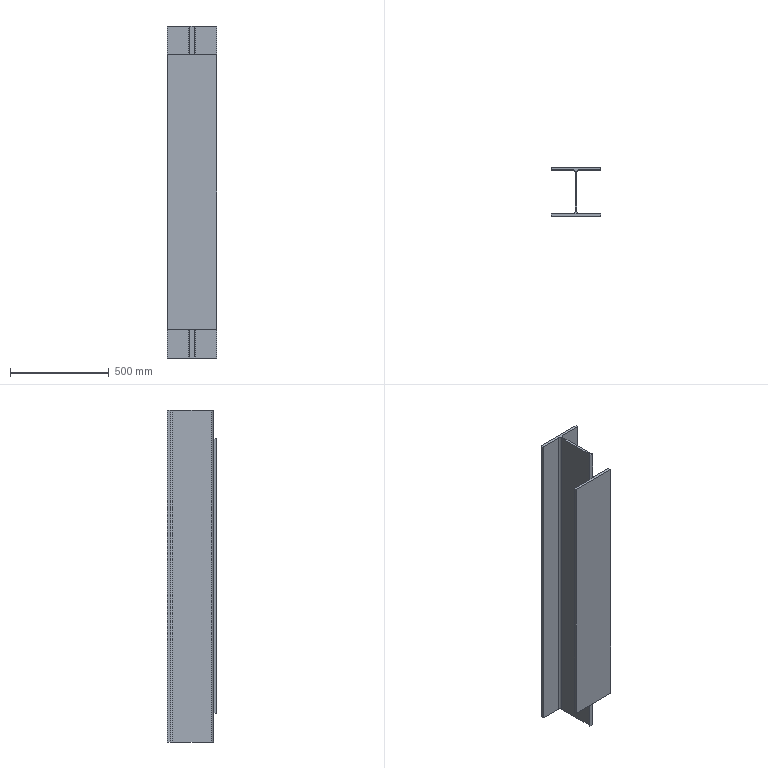Part | SolidWorks | features Extrusion 1, ICE 1 | 1 solid | 22 faces | box 250 x 250 x 1681 mm | volume 14328994 mm3 | plane 18 | cylinder 4 | commonest cylinder face diameters 26 x4
STEP:
#1=CARTESIAN_POINT('',(135.572,16.,0.));
#2=VERTEX_POINT('',#1);
#3=CARTESIAN_POINT('',(129.5,27.,0.));
#4=VERTEX_POINT('',#3);
#5=CARTESIAN_POINT('',(142.5,27.,0.));
#6=DIRECTION('',(0.,0.,-1.));
#7=DIRECTION('',(-1.,0.,0.));
#8=AXIS2_PLACEMENT_3D('',#5,#6,#7);
#9=CIRCLE('',#8,13.);
#10=EDGE_CURVE('',#2,#4,#9,.T.);
#11=ORIENTED_EDGE('',*,*,#10,.F.);
#12=CARTESIAN_POINT('',(114.428,16.,0.));
#13=VERTEX_POINT('',#12);
#14=CARTESIAN_POINT('',(142.5,16.,0.));
#15=DIRECTION('',(-1.,0.,0.));
#16=VECTOR('',#15,1000.);
#17=LINE('',#14,#16);
#18=EDGE_CURVE('',#2,#13,#17,.T.);
#19=ORIENTED_EDGE('',*,*,#18,.T.);
#20=CARTESIAN_POINT('',(120.5,27.,0.));
#21=VERTEX_POINT('',#20);
#22=CARTESIAN_POINT('',(107.5,27.,0.));
#23=DIRECTION('',(0.,0.,-1.));
#24=DIRECTION('',(-1.,0.,0.));
#25=AXIS2_PLACEMENT_3D('',#22,#23,#24);
#26=CIRCLE('',#25,13.);
#27=EDGE_CURVE('',#21,#13,#26,.T.);
#28=ORIENTED_EDGE('',*,*,#27,.F.);
#29=CARTESIAN_POINT('',(120.5,223.,0.));
#30=VERTEX_POINT('',#29);
#31=CARTESIAN_POINT('',(120.5,223.,0.));
#32=DIRECTION('',(0.,-1.,0.));
#33=VECTOR('',#32,1000.);
#34=LINE('',#31,#33);
#35=EDGE_CURVE('',#30,#21,#34,.T.);
#36=ORIENTED_EDGE('',*,*,#35,.F.);
#37=CARTESIAN_POINT('',(107.5,236.,0.));
#38=VERTEX_POINT('',#37);
#39=CARTESIAN_POINT('',(107.5,223.,0.));
#40=DIRECTION('',(0.,0.,-1.));
#41=DIRECTION('',(-1.,0.,0.));
#42=AXIS2_PLACEMENT_3D('',#39,#40,#41);
#43=CIRCLE('',#42,13.);
#44=EDGE_CURVE('',#38,#30,#43,.T.);
#45=ORIENTED_EDGE('',*,*,#44,.F.);
#46=CARTESIAN_POINT('',(0.,236.,0.));
#47=VERTEX_POINT('',#46);
#48=CARTESIAN_POINT('',(0.,236.,0.));
#49=DIRECTION('',(1.,0.,0.));
#50=VECTOR('',#49,1000.);
#51=LINE('',#48,#50);
#52=EDGE_CURVE('',#47,#38,#51,.T.);
#53=ORIENTED_EDGE('',*,*,#52,.F.);
#54=CARTESIAN_POINT('',(0.,250.,0.));
#55=VERTEX_POINT('',#54);
#56=CARTESIAN_POINT('',(0.,250.,0.));
#57=DIRECTION('',(0.,-1.,0.));
#58=VECTOR('',#57,1000.);
#59=LINE('',#56,#58);
#60=EDGE_CURVE('',#55,#47,#59,.T.);
#61=ORIENTED_EDGE('',*,*,#60,.F.);
#62=CARTESIAN_POINT('',(250.,250.,0.));
#63=VERTEX_POINT('',#62);
#64=CARTESIAN_POINT('',(250.,250.,0.));
#65=DIRECTION('',(-1.,0.,0.));
#66=VECTOR('',#65,1000.);
#67=LINE('',#64,#66);
#68=EDGE_CURVE('',#63,#55,#67,.T.);
#69=ORIENTED_EDGE('',*,*,#68,.F.);
#70=CARTESIAN_POINT('',(250.,236.,0.));
#71=VERTEX_POINT('',#70);
#72=CARTESIAN_POINT('',(250.,236.,0.));
#73=DIRECTION('',(0.,1.,0.));
#74=VECTOR('',#73,1000.);
#75=LINE('',#72,#74);
#76=EDGE_CURVE('',#71,#63,#75,.T.);
#77=ORIENTED_EDGE('',*,*,#76,.F.);
#78=CARTESIAN_POINT('',(142.5,236.,0.));
#79=VERTEX_POINT('',#78);
#80=CARTESIAN_POINT('',(142.5,236.,0.));
#81=DIRECTION('',(1.,0.,0.));
#82=VECTOR('',#81,1000.);
#83=LINE('',#80,#82);
#84=EDGE_CURVE('',#79,#71,#83,.T.);
#85=ORIENTED_EDGE('',*,*,#84,.F.);
#86=CARTESIAN_POINT('',(129.5,223.,0.));
#87=VERTEX_POINT('',#86);
#88=CARTESIAN_POINT('',(142.5,223.,0.));
#89=DIRECTION('',(0.,0.,-1.));
#90=DIRECTION('',(-1.,0.,0.));
#91=AXIS2_PLACEMENT_3D('',#88,#89,#90);
#92=CIRCLE('',#91,13.);
#93=EDGE_CURVE('',#87,#79,#92,.T.);
#94=ORIENTED_EDGE('',*,*,#93,.F.);
#95=CARTESIAN_POINT('',(129.5,27.,0.));
#96=DIRECTION('',(0.,1.,0.));
#97=VECTOR('',#96,1000.);
#98=LINE('',#95,#97);
#99=EDGE_CURVE('',#4,#87,#98,.T.);
#100=ORIENTED_EDGE('',*,*,#99,.F.);
#101=EDGE_LOOP('',(#11,#19,#28,#36,#45,#53,#61,#69,#77,#85,#94,#100));
#102=FACE_OUTER_BOUND('',#101,.T.);
#103=CARTESIAN_POINT('',(142.5,27.,0.));
#104=DIRECTION('',(0.,0.,-1.));
#105=DIRECTION('',(-1.,0.,0.));
#106=AXIS2_PLACEMENT_3D('',#103,#104,#105);
#107=PLANE('',#106);
#108=ADVANCED_FACE('',(#102),#107,.T.);
#109=CARTESIAN_POINT('',(0.,14.,1534.5));
#110=VERTEX_POINT('',#109);
#111=CARTESIAN_POINT('',(0.,14.,146.5));
#112=VERTEX_POINT('',#111);
#113=CARTESIAN_POINT('',(0.,14.,1681.));
#114=DIRECTION('',(0.,0.,-1.));
#115=VECTOR('',#114,1000.);
#116=LINE('',#113,#115);
#117=EDGE_CURVE('',#110,#112,#116,.T.);
#118=ORIENTED_EDGE('',*,*,#117,.T.);
#119=CARTESIAN_POINT('',(0.,0.,146.5));
#120=VERTEX_POINT('',#119);
#121=CARTESIAN_POINT('',(0.,16.,146.5));
#122=DIRECTION('',(0.,-1.,0.));
#123=VECTOR('',#122,1000.);
#124=LINE('',#121,#123);
#125=EDGE_CURVE('',#112,#120,#124,.T.);
#126=ORIENTED_EDGE('',*,*,#125,.T.);
#127=CARTESIAN_POINT('',(0.,0.,1534.5));
#128=VERTEX_POINT('',#127);
#129=CARTESIAN_POINT('',(0.,0.,1681.));
#130=DIRECTION('',(0.,0.,-1.));
#131=VECTOR('',#130,1000.);
#132=LINE('',#129,#131);
#133=EDGE_CURVE('',#128,#120,#132,.T.);
#134=ORIENTED_EDGE('',*,*,#133,.F.);
#135=CARTESIAN_POINT('',(0.,16.,1534.5));
#136=DIRECTION('',(0.,-1.,0.));
#137=VECTOR('',#136,1000.);
#138=LINE('',#135,#137);
#139=EDGE_CURVE('',#110,#128,#138,.T.);
#140=ORIENTED_EDGE('',*,*,#139,.F.);
#141=EDGE_LOOP('',(#118,#126,#134,#140));
#142=FACE_OUTER_BOUND('',#141,.T.);
#143=CARTESIAN_POINT('',(0.,14.,1681.));
#144=DIRECTION('',(1.,0.,0.));
#145=DIRECTION('',(0.,1.,0.));
#146=AXIS2_PLACEMENT_3D('',#143,#144,#145);
#147=PLANE('',#146);
#148=ADVANCED_FACE('',(#142),#147,.F.);
#149=ORIENTED_EDGE('',*,*,#133,.T.);
#150=CARTESIAN_POINT('',(250.,0.,146.5));
#151=VERTEX_POINT('',#150);
#152=CARTESIAN_POINT('',(250.,0.,146.5));
#153=DIRECTION('',(-1.,0.,0.));
#154=VECTOR('',#153,1000.);
#155=LINE('',#152,#154);
#156=EDGE_CURVE('',#151,#120,#155,.T.);
#157=ORIENTED_EDGE('',*,*,#156,.F.);
#158=CARTESIAN_POINT('',(250.,0.,1534.5));
#159=VERTEX_POINT('',#158);
#160=CARTESIAN_POINT('',(250.,0.,1681.));
#161=DIRECTION('',(0.,0.,-1.));
#162=VECTOR('',#161,1000.);
#163=LINE('',#160,#162);
#164=EDGE_CURVE('',#159,#151,#163,.T.);
#165=ORIENTED_EDGE('',*,*,#164,.F.);
#166=CARTESIAN_POINT('',(250.,0.,1534.5));
#167=DIRECTION('',(1.,0.,0.));
#168=VECTOR('',#167,1000.);
#169=LINE('',#166,#168);
#170=EDGE_CURVE('',#128,#159,#169,.T.);
#171=ORIENTED_EDGE('',*,*,#170,.F.);
#172=EDGE_LOOP('',(#149,#157,#165,#171));
#173=FACE_OUTER_BOUND('',#172,.T.);
#174=CARTESIAN_POINT('',(0.,0.,1681.));
#175=DIRECTION('',(0.,1.,0.));
#176=DIRECTION('',(-1.,0.,0.));
#177=AXIS2_PLACEMENT_3D('',#174,#175,#176);
#178=PLANE('',#177);
#179=ADVANCED_FACE('',(#173),#178,.F.);
#180=ORIENTED_EDGE('',*,*,#164,.T.);
#181=CARTESIAN_POINT('',(250.,14.,146.5));
#182=VERTEX_POINT('',#181);
#183=CARTESIAN_POINT('',(250.,16.,146.5));
#184=DIRECTION('',(0.,-1.,0.));
#185=VECTOR('',#184,1000.);
#186=LINE('',#183,#185);
#187=EDGE_CURVE('',#182,#151,#186,.T.);
#188=ORIENTED_EDGE('',*,*,#187,.F.);
#189=CARTESIAN_POINT('',(250.,14.,1534.5));
#190=VERTEX_POINT('',#189);
#191=CARTESIAN_POINT('',(250.,14.,1681.));
#192=DIRECTION('',(0.,0.,-1.));
#193=VECTOR('',#192,1000.);
#194=LINE('',#191,#193);
#195=EDGE_CURVE('',#190,#182,#194,.T.);
#196=ORIENTED_EDGE('',*,*,#195,.F.);
#197=CARTESIAN_POINT('',(250.,16.,1534.5));
#198=DIRECTION('',(0.,-1.,0.));
#199=VECTOR('',#198,1000.);
#200=LINE('',#197,#199);
#201=EDGE_CURVE('',#190,#159,#200,.T.);
#202=ORIENTED_EDGE('',*,*,#201,.T.);
#203=EDGE_LOOP('',(#180,#188,#196,#202));
#204=FACE_OUTER_BOUND('',#203,.T.);
#205=CARTESIAN_POINT('',(250.,0.,1681.));
#206=DIRECTION('',(-1.,0.,0.));
#207=DIRECTION('',(0.,0.,1.));
#208=AXIS2_PLACEMENT_3D('',#205,#206,#207);
#209=PLANE('',#208);
#210=ADVANCED_FACE('',(#204),#209,.F.);
#211=ORIENTED_EDGE('',*,*,#195,.T.);
#212=CARTESIAN_POINT('',(142.5,14.,146.5));
#213=VERTEX_POINT('',#212);
#214=CARTESIAN_POINT('',(250.,14.,146.5));
#215=DIRECTION('',(-1.,0.,0.));
#216=VECTOR('',#215,1000.);
#217=LINE('',#214,#216);
#218=EDGE_CURVE('',#182,#213,#217,.T.);
#219=ORIENTED_EDGE('',*,*,#218,.T.);
#220=CARTESIAN_POINT('',(142.5,14.,1534.5));
#221=VERTEX_POINT('',#220);
#222=CARTESIAN_POINT('',(142.5,14.,1681.));
#223=DIRECTION('',(0.,0.,-1.));
#224=VECTOR('',#223,1000.);
#225=LINE('',#222,#224);
#226=EDGE_CURVE('',#221,#213,#225,.T.);
#227=ORIENTED_EDGE('',*,*,#226,.F.);
#228=CARTESIAN_POINT('',(250.,14.,1534.5));
#229=DIRECTION('',(1.,0.,0.));
#230=VECTOR('',#229,1000.);
#231=LINE('',#228,#230);
#232=EDGE_CURVE('',#221,#190,#231,.T.);
#233=ORIENTED_EDGE('',*,*,#232,.T.);
#234=EDGE_LOOP('',(#211,#219,#227,#233));
#235=FACE_OUTER_BOUND('',#234,.T.);
#236=CARTESIAN_POINT('',(250.,14.,1681.));
#237=DIRECTION('',(0.,-1.,0.));
#238=DIRECTION('',(1.,0.,0.));
#239=AXIS2_PLACEMENT_3D('',#236,#237,#238);
#240=PLANE('',#239);
#241=ADVANCED_FACE('',(#235),#240,.F.);
#242=ORIENTED_EDGE('',*,*,#226,.T.);
#243=CARTESIAN_POINT('',(135.572,16.,146.5));
#244=VERTEX_POINT('',#243);
#245=CARTESIAN_POINT('',(142.5,27.,146.5));
#246=DIRECTION('',(0.,0.,-1.));
#247=DIRECTION('',(1.,0.,0.));
#248=AXIS2_PLACEMENT_3D('',#245,#246,#247);
#249=CIRCLE('',#248,13.);
#250=EDGE_CURVE('',#213,#244,#249,.T.);
#251=ORIENTED_EDGE('',*,*,#250,.T.);
#252=CARTESIAN_POINT('',(135.572,16.,1681.));
#253=DIRECTION('',(0.,0.,1.));
#254=VECTOR('',#253,1000.);
#255=LINE('',#252,#254);
#256=EDGE_CURVE('',#2,#244,#255,.T.);
#257=ORIENTED_EDGE('',*,*,#256,.F.);
#258=ORIENTED_EDGE('',*,*,#10,.T.);
#259=CARTESIAN_POINT('',(129.5,27.,1681.));
#260=VERTEX_POINT('',#259);
#261=CARTESIAN_POINT('',(129.5,27.,1681.));
#262=DIRECTION('',(0.,0.,-1.));
#263=VECTOR('',#262,1000.);
#264=LINE('',#261,#263);
#265=EDGE_CURVE('',#260,#4,#264,.T.);
#266=ORIENTED_EDGE('',*,*,#265,.F.);
#267=CARTESIAN_POINT('',(135.572,16.,1681.));
#268=VERTEX_POINT('',#267);
#269=CARTESIAN_POINT('',(142.5,27.,1681.));
#270=DIRECTION('',(0.,0.,-1.));
#271=DIRECTION('',(-1.,0.,0.));
#272=AXIS2_PLACEMENT_3D('',#269,#270,#271);
#273=CIRCLE('',#272,13.);
#274=EDGE_CURVE('',#268,#260,#273,.T.);
#275=ORIENTED_EDGE('',*,*,#274,.F.);
#276=CARTESIAN_POINT('',(135.572,16.,1534.5));
#277=VERTEX_POINT('',#276);
#278=CARTESIAN_POINT('',(135.572,16.,1681.));
#279=DIRECTION('',(0.,0.,-1.));
#280=VECTOR('',#279,1000.);
#281=LINE('',#278,#280);
#282=EDGE_CURVE('',#268,#277,#281,.T.);
#283=ORIENTED_EDGE('',*,*,#282,.T.);
#284=CARTESIAN_POINT('',(142.5,27.,1534.5));
#285=DIRECTION('',(0.,0.,1.));
#286=DIRECTION('',(-1.,0.,0.));
#287=AXIS2_PLACEMENT_3D('',#284,#285,#286);
#288=CIRCLE('',#287,13.);
#289=EDGE_CURVE('',#277,#221,#288,.T.);
#290=ORIENTED_EDGE('',*,*,#289,.T.);
#291=EDGE_LOOP('',(#242,#251,#257,#258,#266,#275,#283,#290));
#292=FACE_OUTER_BOUND('',#291,.T.);
#293=CARTESIAN_POINT('',(142.5,27.,1681.));
#294=DIRECTION('',(0.,0.,-1.));
#295=DIRECTION('',(-1.,0.,0.));
#296=AXIS2_PLACEMENT_3D('',#293,#294,#295);
#297=CYLINDRICAL_SURFACE('',#296,13.);
#298=ADVANCED_FACE('',(#292),#297,.F.);
#299=ORIENTED_EDGE('',*,*,#99,.T.);
#300=CARTESIAN_POINT('',(129.5,223.,1681.));
#301=VERTEX_POINT('',#300);
#302=CARTESIAN_POINT('',(129.5,223.,1681.));
#303=DIRECTION('',(0.,0.,-1.));
#304=VECTOR('',#303,1000.);
#305=LINE('',#302,#304);
#306=EDGE_CURVE('',#301,#87,#305,.T.);
#307=ORIENTED_EDGE('',*,*,#306,.F.);
#308=CARTESIAN_POINT('',(129.5,27.,1681.));
#309=DIRECTION('',(0.,1.,0.));
#310=VECTOR('',#309,1000.);
#311=LINE('',#308,#310);
#312=EDGE_CURVE('',#260,#301,#311,.T.);
#313=ORIENTED_EDGE('',*,*,#312,.F.);
#314=ORIENTED_EDGE('',*,*,#265,.T.);
#315=EDGE_LOOP('',(#299,#307,#313,#314));
#316=FACE_OUTER_BOUND('',#315,.T.);
#317=CARTESIAN_POINT('',(129.5,27.,1681.));
#318=DIRECTION('',(-1.,0.,0.));
#319=DIRECTION('',(0.,-1.,0.));
#320=AXIS2_PLACEMENT_3D('',#317,#318,#319);
#321=PLANE('',#320);
#322=ADVANCED_FACE('',(#316),#321,.F.);
#323=ORIENTED_EDGE('',*,*,#93,.T.);
#324=CARTESIAN_POINT('',(142.5,236.,1681.));
#325=VERTEX_POINT('',#324);
#326=CARTESIAN_POINT('',(142.5,236.,1681.));
#327=DIRECTION('',(0.,0.,-1.));
#328=VECTOR('',#327,1000.);
#329=LINE('',#326,#328);
#330=EDGE_CURVE('',#325,#79,#329,.T.);
#331=ORIENTED_EDGE('',*,*,#330,.F.);
#332=CARTESIAN_POINT('',(142.5,223.,1681.));
#333=DIRECTION('',(0.,0.,-1.));
#334=DIRECTION('',(-1.,0.,0.));
#335=AXIS2_PLACEMENT_3D('',#332,#333,#334);
#336=CIRCLE('',#335,13.);
#337=EDGE_CURVE('',#301,#325,#336,.T.);
#338=ORIENTED_EDGE('',*,*,#337,.F.);
#339=ORIENTED_EDGE('',*,*,#306,.T.);
#340=EDGE_LOOP('',(#323,#331,#338,#339));
#341=FACE_OUTER_BOUND('',#340,.T.);
#342=CARTESIAN_POINT('',(142.5,223.,1681.));
#343=DIRECTION('',(0.,0.,-1.));
#344=DIRECTION('',(-1.,0.,0.));
#345=AXIS2_PLACEMENT_3D('',#342,#343,#344);
#346=CYLINDRICAL_SURFACE('',#345,13.);
#347=ADVANCED_FACE('',(#341),#346,.F.);
#348=ORIENTED_EDGE('',*,*,#84,.T.);
#349=CARTESIAN_POINT('',(250.,236.,1681.));
#350=VERTEX_POINT('',#349);
#351=CARTESIAN_POINT('',(250.,236.,1681.));
#352=DIRECTION('',(0.,0.,-1.));
#353=VECTOR('',#352,1000.);
#354=LINE('',#351,#353);
#355=EDGE_CURVE('',#350,#71,#354,.T.);
#356=ORIENTED_EDGE('',*,*,#355,.F.);
#357=CARTESIAN_POINT('',(142.5,236.,1681.));
#358=DIRECTION('',(1.,0.,0.));
#359=VECTOR('',#358,1000.);
#360=LINE('',#357,#359);
#361=EDGE_CURVE('',#325,#350,#360,.T.);
#362=ORIENTED_EDGE('',*,*,#361,.F.);
#363=ORIENTED_EDGE('',*,*,#330,.T.);
#364=EDGE_LOOP('',(#348,#356,#362,#363));
#365=FACE_OUTER_BOUND('',#364,.T.);
#366=CARTESIAN_POINT('',(142.5,236.,1681.));
#367=DIRECTION('',(0.,1.,0.));
#368=DIRECTION('',(0.,0.,1.));
#369=AXIS2_PLACEMENT_3D('',#366,#367,#368);
#370=PLANE('',#369);
#371=ADVANCED_FACE('',(#365),#370,.F.);
#372=ORIENTED_EDGE('',*,*,#76,.T.);
#373=CARTESIAN_POINT('',(250.,250.,1681.));
#374=VERTEX_POINT('',#373);
#375=CARTESIAN_POINT('',(250.,250.,1681.));
#376=DIRECTION('',(0.,0.,-1.));
#377=VECTOR('',#376,1000.);
#378=LINE('',#375,#377);
#379=EDGE_CURVE('',#374,#63,#378,.T.);
#380=ORIENTED_EDGE('',*,*,#379,.F.);
#381=CARTESIAN_POINT('',(250.,236.,1681.));
#382=DIRECTION('',(0.,1.,0.));
#383=VECTOR('',#382,1000.);
#384=LINE('',#381,#383);
#385=EDGE_CURVE('',#350,#374,#384,.T.);
#386=ORIENTED_EDGE('',*,*,#385,.F.);
#387=ORIENTED_EDGE('',*,*,#355,.T.);
#388=EDGE_LOOP('',(#372,#380,#386,#387));
#389=FACE_OUTER_BOUND('',#388,.T.);
#390=CARTESIAN_POINT('',(250.,236.,1681.));
#391=DIRECTION('',(-1.,0.,0.));
#392=DIRECTION('',(0.,0.,1.));
#393=AXIS2_PLACEMENT_3D('',#390,#391,#392);
#394=PLANE('',#393);
#395=ADVANCED_FACE('',(#389),#394,.F.);
#396=ORIENTED_EDGE('',*,*,#68,.T.);
#397=CARTESIAN_POINT('',(0.,250.,1681.));
#398=VERTEX_POINT('',#397);
#399=CARTESIAN_POINT('',(0.,250.,1681.));
#400=DIRECTION('',(0.,0.,-1.));
#401=VECTOR('',#400,1000.);
#402=LINE('',#399,#401);
#403=EDGE_CURVE('',#398,#55,#402,.T.);
#404=ORIENTED_EDGE('',*,*,#403,.F.);
#405=CARTESIAN_POINT('',(250.,250.,1681.));
#406=DIRECTION('',(-1.,0.,0.));
#407=VECTOR('',#406,1000.);
#408=LINE('',#405,#407);
#409=EDGE_CURVE('',#374,#398,#408,.T.);
#410=ORIENTED_EDGE('',*,*,#409,.F.);
#411=ORIENTED_EDGE('',*,*,#379,.T.);
#412=EDGE_LOOP('',(#396,#404,#410,#411));
#413=FACE_OUTER_BOUND('',#412,.T.);
#414=CARTESIAN_POINT('',(250.,250.,1681.));
#415=DIRECTION('',(0.,-1.,0.));
#416=DIRECTION('',(0.,0.,-1.));
#417=AXIS2_PLACEMENT_3D('',#414,#415,#416);
#418=PLANE('',#417);
#419=ADVANCED_FACE('',(#413),#418,.F.);
#420=ORIENTED_EDGE('',*,*,#60,.T.);
#421=CARTESIAN_POINT('',(0.,236.,1681.));
#422=VERTEX_POINT('',#421);
#423=CARTESIAN_POINT('',(0.,236.,1681.));
#424=DIRECTION('',(0.,0.,-1.));
#425=VECTOR('',#424,1000.);
#426=LINE('',#423,#425);
#427=EDGE_CURVE('',#422,#47,#426,.T.);
#428=ORIENTED_EDGE('',*,*,#427,.F.);
#429=CARTESIAN_POINT('',(0.,250.,1681.));
#430=DIRECTION('',(0.,-1.,0.));
#431=VECTOR('',#430,1000.);
#432=LINE('',#429,#431);
#433=EDGE_CURVE('',#398,#422,#432,.T.);
#434=ORIENTED_EDGE('',*,*,#433,.F.);
#435=ORIENTED_EDGE('',*,*,#403,.T.);
#436=EDGE_LOOP('',(#420,#428,#434,#435));
#437=FACE_OUTER_BOUND('',#436,.T.);
#438=CARTESIAN_POINT('',(0.,250.,1681.));
#439=DIRECTION('',(1.,0.,0.));
#440=DIRECTION('',(0.,1.,0.));
#441=AXIS2_PLACEMENT_3D('',#438,#439,#440);
#442=PLANE('',#441);
#443=ADVANCED_FACE('',(#437),#442,.F.);
#444=ORIENTED_EDGE('',*,*,#52,.T.);
#445=CARTESIAN_POINT('',(107.5,236.,1681.));
#446=VERTEX_POINT('',#445);
#447=CARTESIAN_POINT('',(107.5,236.,1681.));
#448=DIRECTION('',(0.,0.,-1.));
#449=VECTOR('',#448,1000.);
#450=LINE('',#447,#449);
#451=EDGE_CURVE('',#446,#38,#450,.T.);
#452=ORIENTED_EDGE('',*,*,#451,.F.);
#453=CARTESIAN_POINT('',(0.,236.,1681.));
#454=DIRECTION('',(1.,0.,0.));
#455=VECTOR('',#454,1000.);
#456=LINE('',#453,#455);
#457=EDGE_CURVE('',#422,#446,#456,.T.);
#458=ORIENTED_EDGE('',*,*,#457,.F.);
#459=ORIENTED_EDGE('',*,*,#427,.T.);
#460=EDGE_LOOP('',(#444,#452,#458,#459));
#461=FACE_OUTER_BOUND('',#460,.T.);
#462=CARTESIAN_POINT('',(0.,236.,1681.));
#463=DIRECTION('',(0.,1.,0.));
#464=DIRECTION('',(-1.,0.,0.));
#465=AXIS2_PLACEMENT_3D('',#462,#463,#464);
#466=PLANE('',#465);
#467=ADVANCED_FACE('',(#461),#466,.F.);
#468=ORIENTED_EDGE('',*,*,#44,.T.);
#469=CARTESIAN_POINT('',(120.5,223.,1681.));
#470=VERTEX_POINT('',#469);
#471=CARTESIAN_POINT('',(120.5,223.,1681.));
#472=DIRECTION('',(0.,0.,-1.));
#473=VECTOR('',#472,1000.);
#474=LINE('',#471,#473);
#475=EDGE_CURVE('',#470,#30,#474,.T.);
#476=ORIENTED_EDGE('',*,*,#475,.F.);
#477=CARTESIAN_POINT('',(107.5,223.,1681.));
#478=DIRECTION('',(0.,0.,-1.));
#479=DIRECTION('',(-1.,0.,0.));
#480=AXIS2_PLACEMENT_3D('',#477,#478,#479);
#481=CIRCLE('',#480,13.);
#482=EDGE_CURVE('',#446,#470,#481,.T.);
#483=ORIENTED_EDGE('',*,*,#482,.F.);
#484=ORIENTED_EDGE('',*,*,#451,.T.);
#485=EDGE_LOOP('',(#468,#476,#483,#484));
#486=FACE_OUTER_BOUND('',#485,.T.);
#487=CARTESIAN_POINT('',(107.5,223.,1681.));
#488=DIRECTION('',(0.,0.,-1.));
#489=DIRECTION('',(-1.,0.,0.));
#490=AXIS2_PLACEMENT_3D('',#487,#488,#489);
#491=CYLINDRICAL_SURFACE('',#490,13.);
#492=ADVANCED_FACE('',(#486),#491,.F.);
#493=ORIENTED_EDGE('',*,*,#35,.T.);
#494=CARTESIAN_POINT('',(120.5,27.,1681.));
#495=VERTEX_POINT('',#494);
#496=CARTESIAN_POINT('',(120.5,27.,1681.));
#497=DIRECTION('',(0.,0.,-1.));
#498=VECTOR('',#497,1000.);
#499=LINE('',#496,#498);
#500=EDGE_CURVE('',#495,#21,#499,.T.);
#501=ORIENTED_EDGE('',*,*,#500,.F.);
#502=CARTESIAN_POINT('',(120.5,223.,1681.));
#503=DIRECTION('',(0.,-1.,0.));
#504=VECTOR('',#503,1000.);
#505=LINE('',#502,#504);
#506=EDGE_CURVE('',#470,#495,#505,.T.);
#507=ORIENTED_EDGE('',*,*,#506,.F.);
#508=ORIENTED_EDGE('',*,*,#475,.T.);
#509=EDGE_LOOP('',(#493,#501,#507,#508));
#510=FACE_OUTER_BOUND('',#509,.T.);
#511=CARTESIAN_POINT('',(120.5,223.,1681.));
#512=DIRECTION('',(1.,0.,0.));
#513=DIRECTION('',(0.,1.,0.));
#514=AXIS2_PLACEMENT_3D('',#511,#512,#513);
#515=PLANE('',#514);
#516=ADVANCED_FACE('',(#510),#515,.F.);
#517=CARTESIAN_POINT('',(114.428,16.,146.5));
#518=VERTEX_POINT('',#517);
#519=CARTESIAN_POINT('',(114.428,16.,1681.));
#520=DIRECTION('',(0.,0.,-1.));
#521=VECTOR('',#520,1000.);
#522=LINE('',#519,#521);
#523=EDGE_CURVE('',#518,#13,#522,.T.);
#524=ORIENTED_EDGE('',*,*,#523,.F.);
#525=CARTESIAN_POINT('',(107.5,14.,146.5));
#526=VERTEX_POINT('',#525);
#527=CARTESIAN_POINT('',(107.5,27.,146.5));
#528=DIRECTION('',(0.,0.,-1.));
#529=DIRECTION('',(1.,0.,0.));
#530=AXIS2_PLACEMENT_3D('',#527,#528,#529);
#531=CIRCLE('',#530,13.);
#532=EDGE_CURVE('',#518,#526,#531,.T.);
#533=ORIENTED_EDGE('',*,*,#532,.T.);
#534=CARTESIAN_POINT('',(107.5,14.,1534.5));
#535=VERTEX_POINT('',#534);
#536=CARTESIAN_POINT('',(107.5,14.,1681.));
#537=DIRECTION('',(0.,0.,-1.));
#538=VECTOR('',#537,1000.);
#539=LINE('',#536,#538);
#540=EDGE_CURVE('',#535,#526,#539,.T.);
#541=ORIENTED_EDGE('',*,*,#540,.F.);
#542=CARTESIAN_POINT('',(114.428,16.,1534.5));
#543=VERTEX_POINT('',#542);
#544=CARTESIAN_POINT('',(107.5,27.,1534.5));
#545=DIRECTION('',(0.,0.,1.));
#546=DIRECTION('',(-1.,0.,0.));
#547=AXIS2_PLACEMENT_3D('',#544,#545,#546);
#548=CIRCLE('',#547,13.);
#549=EDGE_CURVE('',#535,#543,#548,.T.);
#550=ORIENTED_EDGE('',*,*,#549,.T.);
#551=CARTESIAN_POINT('',(114.428,16.,1681.));
#552=VERTEX_POINT('',#551);
#553=CARTESIAN_POINT('',(114.428,16.,1681.));
#554=DIRECTION('',(0.,0.,1.));
#555=VECTOR('',#554,1000.);
#556=LINE('',#553,#555);
#557=EDGE_CURVE('',#543,#552,#556,.T.);
#558=ORIENTED_EDGE('',*,*,#557,.T.);
#559=CARTESIAN_POINT('',(107.5,27.,1681.));
#560=DIRECTION('',(0.,0.,-1.));
#561=DIRECTION('',(-1.,0.,0.));
#562=AXIS2_PLACEMENT_3D('',#559,#560,#561);
#563=CIRCLE('',#562,13.);
#564=EDGE_CURVE('',#495,#552,#563,.T.);
#565=ORIENTED_EDGE('',*,*,#564,.F.);
#566=ORIENTED_EDGE('',*,*,#500,.T.);
#567=ORIENTED_EDGE('',*,*,#27,.T.);
#568=EDGE_LOOP('',(#524,#533,#541,#550,#558,#565,#566,#567));
#569=FACE_OUTER_BOUND('',#568,.T.);
#570=CARTESIAN_POINT('',(107.5,27.,1681.));
#571=DIRECTION('',(0.,0.,-1.));
#572=DIRECTION('',(-1.,0.,0.));
#573=AXIS2_PLACEMENT_3D('',#570,#571,#572);
#574=CYLINDRICAL_SURFACE('',#573,13.);
#575=ADVANCED_FACE('',(#569),#574,.F.);
#576=ORIENTED_EDGE('',*,*,#540,.T.);
#577=CARTESIAN_POINT('',(107.5,14.,146.5));
#578=DIRECTION('',(-1.,0.,0.));
#579=VECTOR('',#578,1000.);
#580=LINE('',#577,#579);
#581=EDGE_CURVE('',#526,#112,#580,.T.);
#582=ORIENTED_EDGE('',*,*,#581,.T.);
#583=ORIENTED_EDGE('',*,*,#117,.F.);
#584=CARTESIAN_POINT('',(107.5,14.,1534.5));
#585=DIRECTION('',(1.,0.,0.));
#586=VECTOR('',#585,1000.);
#587=LINE('',#584,#586);
#588=EDGE_CURVE('',#110,#535,#587,.T.);
#589=ORIENTED_EDGE('',*,*,#588,.T.);
#590=EDGE_LOOP('',(#576,#582,#583,#589));
#591=FACE_OUTER_BOUND('',#590,.T.);
#592=CARTESIAN_POINT('',(107.5,14.,1681.));
#593=DIRECTION('',(0.,-1.,0.));
#594=DIRECTION('',(1.,0.,0.));
#595=AXIS2_PLACEMENT_3D('',#592,#593,#594);
#596=PLANE('',#595);
#597=ADVANCED_FACE('',(#591),#596,.F.);
#598=ORIENTED_EDGE('',*,*,#564,.T.);
#599=CARTESIAN_POINT('',(142.5,16.,1681.));
#600=DIRECTION('',(1.,0.,0.));
#601=VECTOR('',#600,1000.);
#602=LINE('',#599,#601);
#603=EDGE_CURVE('',#552,#268,#602,.T.);
#604=ORIENTED_EDGE('',*,*,#603,.T.);
#605=ORIENTED_EDGE('',*,*,#274,.T.);
#606=ORIENTED_EDGE('',*,*,#312,.T.);
#607=ORIENTED_EDGE('',*,*,#337,.T.);
#608=ORIENTED_EDGE('',*,*,#361,.T.);
#609=ORIENTED_EDGE('',*,*,#385,.T.);
#610=ORIENTED_EDGE('',*,*,#409,.T.);
#611=ORIENTED_EDGE('',*,*,#433,.T.);
#612=ORIENTED_EDGE('',*,*,#457,.T.);
#613=ORIENTED_EDGE('',*,*,#482,.T.);
#614=ORIENTED_EDGE('',*,*,#506,.T.);
#615=EDGE_LOOP('',(#598,#604,#605,#606,#607,#608,#609,#610,#611,#612,#613,#614));
#616=FACE_OUTER_BOUND('',#615,.T.);
#617=CARTESIAN_POINT('',(142.5,27.,1681.));
#618=DIRECTION('',(0.,0.,-1.));
#619=DIRECTION('',(-1.,0.,0.));
#620=AXIS2_PLACEMENT_3D('',#617,#618,#619);
#621=PLANE('',#620);
#622=ADVANCED_FACE('',(#616),#621,.F.);
#623=ORIENTED_EDGE('',*,*,#187,.T.);
#624=ORIENTED_EDGE('',*,*,#156,.T.);
#625=ORIENTED_EDGE('',*,*,#125,.F.);
#626=ORIENTED_EDGE('',*,*,#581,.F.);
#627=ORIENTED_EDGE('',*,*,#532,.F.);
#628=CARTESIAN_POINT('',(250.,16.,146.5));
#629=DIRECTION('',(-1.,0.,0.));
#630=VECTOR('',#629,1000.);
#631=LINE('',#628,#630);
#632=EDGE_CURVE('',#244,#518,#631,.T.);
#633=ORIENTED_EDGE('',*,*,#632,.F.);
#634=ORIENTED_EDGE('',*,*,#250,.F.);
#635=ORIENTED_EDGE('',*,*,#218,.F.);
#636=EDGE_LOOP('',(#623,#624,#625,#626,#627,#633,#634,#635));
#637=FACE_OUTER_BOUND('',#636,.T.);
#638=CARTESIAN_POINT('',(250.,16.,146.5));
#639=DIRECTION('',(0.,0.,1.));
#640=DIRECTION('',(1.,0.,0.));
#641=AXIS2_PLACEMENT_3D('',#638,#639,#640);
#642=PLANE('',#641);
#643=ADVANCED_FACE('',(#637),#642,.F.);
#644=ORIENTED_EDGE('',*,*,#256,.T.);
#645=ORIENTED_EDGE('',*,*,#632,.T.);
#646=ORIENTED_EDGE('',*,*,#523,.T.);
#647=ORIENTED_EDGE('',*,*,#18,.F.);
#648=EDGE_LOOP('',(#644,#645,#646,#647));
#649=FACE_OUTER_BOUND('',#648,.T.);
#650=CARTESIAN_POINT('',(0.,16.,0.));
#651=DIRECTION('',(0.,-1.,0.));
#652=DIRECTION('',(1.,0.,0.));
#653=AXIS2_PLACEMENT_3D('',#650,#651,#652);
#654=PLANE('',#653);
#655=ADVANCED_FACE('',(#649),#654,.T.);
#656=ORIENTED_EDGE('',*,*,#289,.F.);
#657=CARTESIAN_POINT('',(250.,16.,1534.5));
#658=DIRECTION('',(1.,0.,0.));
#659=VECTOR('',#658,1000.);
#660=LINE('',#657,#659);
#661=EDGE_CURVE('',#543,#277,#660,.T.);
#662=ORIENTED_EDGE('',*,*,#661,.F.);
#663=ORIENTED_EDGE('',*,*,#549,.F.);
#664=ORIENTED_EDGE('',*,*,#588,.F.);
#665=ORIENTED_EDGE('',*,*,#139,.T.);
#666=ORIENTED_EDGE('',*,*,#170,.T.);
#667=ORIENTED_EDGE('',*,*,#201,.F.);
#668=ORIENTED_EDGE('',*,*,#232,.F.);
#669=EDGE_LOOP('',(#656,#662,#663,#664,#665,#666,#667,#668));
#670=FACE_OUTER_BOUND('',#669,.T.);
#671=CARTESIAN_POINT('',(250.,16.,1534.5));
#672=DIRECTION('',(0.,0.,-1.));
#673=DIRECTION('',(-1.,0.,0.));
#674=AXIS2_PLACEMENT_3D('',#671,#672,#673);
#675=PLANE('',#674);
#676=ADVANCED_FACE('',(#670),#675,.F.);
#677=ORIENTED_EDGE('',*,*,#603,.F.);
#678=ORIENTED_EDGE('',*,*,#557,.F.);
#679=ORIENTED_EDGE('',*,*,#661,.T.);
#680=ORIENTED_EDGE('',*,*,#282,.F.);
#681=EDGE_LOOP('',(#677,#678,#679,#680));
#682=FACE_OUTER_BOUND('',#681,.T.);
#683=CARTESIAN_POINT('',(0.,16.,0.));
#684=DIRECTION('',(0.,1.,0.));
#685=DIRECTION('',(-1.,0.,0.));
#686=AXIS2_PLACEMENT_3D('',#683,#684,#685);
#687=PLANE('',#686);
#688=ADVANCED_FACE('',(#682),#687,.F.);
#689=CLOSED_SHELL('',(#108,#148,#179,#210,#241,#298,#322,#347,#371,#395,#419,#443,#467,#492,#516,#575,#597,#622,#643,#655,#676,#688));
#690=MANIFOLD_SOLID_BREP('',#689);
#691=CARTESIAN_POINT('',(0.,0.,0.));
#692=DIRECTION('',(0.,0.,1.));
#693=DIRECTION('',(1.,0.,0.));
#694=AXIS2_PLACEMENT_3D('',#691,#692,#693);
#695=(LENGTH_UNIT()NAMED_UNIT(*)SI_UNIT(.MILLI.,.METRE.));
#696=UNCERTAINTY_MEASURE_WITH_UNIT(LENGTH_MEASURE(0.00001),#695,'','');
#697=(NAMED_UNIT(*)PLANE_ANGLE_UNIT()SI_UNIT($,.RADIAN.));
#698=(NAMED_UNIT(*)SI_UNIT($,.STERADIAN.)SOLID_ANGLE_UNIT());
#699=(GEOMETRIC_REPRESENTATION_CONTEXT(3)GLOBAL_UNCERTAINTY_ASSIGNED_CONTEXT((#696))GLOBAL_UNIT_ASSIGNED_CONTEXT((#695,#697,#698))REPRESENTATION_CONTEXT('',''));
#700=ADVANCED_BREP_SHAPE_REPRESENTATION('',(#690,#694),#699);